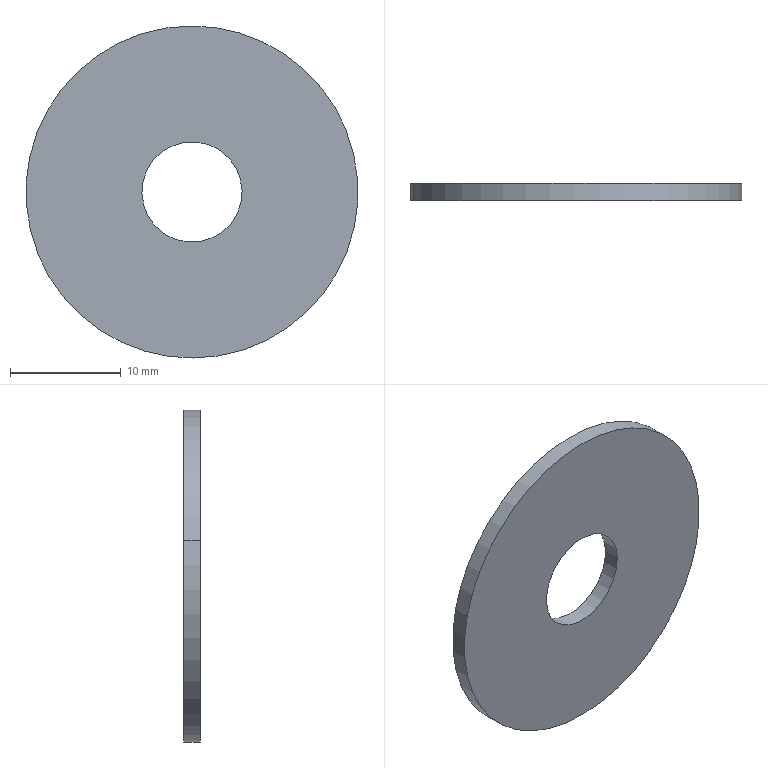Part | STEP file | 2026.6.15-Main Assembly图.sldasm-Part-204 | 1 solid | 6 faces | box 30 x 1.5 x 30 mm | volume 963.585 mm3 | cylinder 4 | plane 2 | commonest cylinder face diameters 9.06 x2 30 x2
STEP:
#1=CARTESIAN_POINT('',(-1645.889,1406.264,3355.366));
#2=VERTEX_POINT('',#1);
#3=CARTESIAN_POINT('',(-1616.588,1406.264,3348.928));
#4=VERTEX_POINT('',#3);
#5=CARTESIAN_POINT('',(-1631.238,1406.264,3352.147));
#6=DIRECTION('',(0.,-1.,0.));
#7=DIRECTION('',(-0.9767,0.,0.2146));
#8=AXIS2_PLACEMENT_3D('',#5,#6,#7);
#9=CIRCLE('',#8,15.);
#10=EDGE_CURVE('',#2,#4,#9,.T.);
#11=ORIENTED_EDGE('',*,*,#10,.F.);
#12=CARTESIAN_POINT('',(-1631.238,1406.264,3352.147));
#13=DIRECTION('',(0.,-1.,0.));
#14=DIRECTION('',(-0.9767,0.,0.2146));
#15=AXIS2_PLACEMENT_3D('',#12,#13,#14);
#16=CIRCLE('',#15,15.);
#17=EDGE_CURVE('',#4,#2,#16,.T.);
#18=ORIENTED_EDGE('',*,*,#17,.F.);
#19=EDGE_LOOP('',(#11,#18));
#20=FACE_OUTER_BOUND('',#19,.T.);
#21=CARTESIAN_POINT('',(-1635.663,1406.264,3353.119));
#22=VERTEX_POINT('',#21);
#23=CARTESIAN_POINT('',(-1626.814,1406.264,3351.175));
#24=VERTEX_POINT('',#23);
#25=CARTESIAN_POINT('',(-1631.238,1406.264,3352.147));
#26=DIRECTION('',(0.,-1.,0.));
#27=DIRECTION('',(-0.9767,0.,0.2146));
#28=AXIS2_PLACEMENT_3D('',#25,#26,#27);
#29=CIRCLE('',#28,4.53);
#30=EDGE_CURVE('',#22,#24,#29,.T.);
#31=ORIENTED_EDGE('',*,*,#30,.T.);
#32=CARTESIAN_POINT('',(-1631.238,1406.264,3352.147));
#33=DIRECTION('',(0.,-1.,0.));
#34=DIRECTION('',(-0.9767,0.,0.2146));
#35=AXIS2_PLACEMENT_3D('',#32,#33,#34);
#36=CIRCLE('',#35,4.53);
#37=EDGE_CURVE('',#24,#22,#36,.T.);
#38=ORIENTED_EDGE('',*,*,#37,.T.);
#39=EDGE_LOOP('',(#31,#38));
#40=FACE_BOUND('',#39,.T.);
#41=CARTESIAN_POINT('',(-1631.238,1406.264,3352.147));
#42=DIRECTION('',(0.,-1.,0.));
#43=DIRECTION('',(0.,0.,-1.));
#44=AXIS2_PLACEMENT_3D('',#41,#42,#43);
#45=PLANE('',#44);
#46=ADVANCED_FACE('',(#20,#40),#45,.F.);
#47=CARTESIAN_POINT('',(-1616.588,1404.764,3348.928));
#48=VERTEX_POINT('',#47);
#49=CARTESIAN_POINT('',(-1616.588,1404.764,3348.928));
#50=DIRECTION('',(0.,-1.,0.));
#51=VECTOR('',#50,1000.);
#52=LINE('',#49,#51);
#53=EDGE_CURVE('',#4,#48,#52,.T.);
#54=ORIENTED_EDGE('',*,*,#53,.T.);
#55=CARTESIAN_POINT('',(-1645.889,1404.764,3355.366));
#56=VERTEX_POINT('',#55);
#57=CARTESIAN_POINT('',(-1631.238,1404.764,3352.147));
#58=DIRECTION('',(0.,-1.,0.));
#59=DIRECTION('',(-0.9767,0.,0.2146));
#60=AXIS2_PLACEMENT_3D('',#57,#58,#59);
#61=CIRCLE('',#60,15.);
#62=EDGE_CURVE('',#56,#48,#61,.T.);
#63=ORIENTED_EDGE('',*,*,#62,.F.);
#64=CARTESIAN_POINT('',(-1645.889,1404.764,3355.366));
#65=DIRECTION('',(0.,-1.,0.));
#66=VECTOR('',#65,1000.);
#67=LINE('',#64,#66);
#68=EDGE_CURVE('',#2,#56,#67,.T.);
#69=ORIENTED_EDGE('',*,*,#68,.F.);
#70=ORIENTED_EDGE('',*,*,#10,.T.);
#71=EDGE_LOOP('',(#54,#63,#69,#70));
#72=FACE_OUTER_BOUND('',#71,.T.);
#73=CARTESIAN_POINT('',(-1631.238,1404.764,3352.147));
#74=DIRECTION('',(0.,1.,0.));
#75=DIRECTION('',(0.9767,0.,-0.2146));
#76=AXIS2_PLACEMENT_3D('',#73,#74,#75);
#77=CYLINDRICAL_SURFACE('',#76,15.);
#78=ADVANCED_FACE('',(#72),#77,.T.);
#79=CARTESIAN_POINT('',(-1626.814,1404.764,3351.175));
#80=VERTEX_POINT('',#79);
#81=CARTESIAN_POINT('',(-1626.814,1404.764,3351.175));
#82=DIRECTION('',(0.,-1.,0.));
#83=VECTOR('',#82,1000.);
#84=LINE('',#81,#83);
#85=EDGE_CURVE('',#24,#80,#84,.T.);
#86=ORIENTED_EDGE('',*,*,#85,.T.);
#87=CARTESIAN_POINT('',(-1635.663,1404.764,3353.119));
#88=VERTEX_POINT('',#87);
#89=CARTESIAN_POINT('',(-1631.238,1404.764,3352.147));
#90=DIRECTION('',(0.,1.,0.));
#91=DIRECTION('',(-0.9767,0.,0.2146));
#92=AXIS2_PLACEMENT_3D('',#89,#90,#91);
#93=CIRCLE('',#92,4.53);
#94=EDGE_CURVE('',#88,#80,#93,.T.);
#95=ORIENTED_EDGE('',*,*,#94,.F.);
#96=CARTESIAN_POINT('',(-1635.663,1404.764,3353.119));
#97=DIRECTION('',(0.,-1.,0.));
#98=VECTOR('',#97,1000.);
#99=LINE('',#96,#98);
#100=EDGE_CURVE('',#22,#88,#99,.T.);
#101=ORIENTED_EDGE('',*,*,#100,.F.);
#102=ORIENTED_EDGE('',*,*,#37,.F.);
#103=EDGE_LOOP('',(#86,#95,#101,#102));
#104=FACE_OUTER_BOUND('',#103,.T.);
#105=CARTESIAN_POINT('',(-1631.238,1404.764,3352.147));
#106=DIRECTION('',(0.,1.,0.));
#107=DIRECTION('',(0.9767,0.,-0.2146));
#108=AXIS2_PLACEMENT_3D('',#105,#106,#107);
#109=CYLINDRICAL_SURFACE('',#108,4.53);
#110=ADVANCED_FACE('',(#104),#109,.F.);
#111=ORIENTED_EDGE('',*,*,#62,.T.);
#112=CARTESIAN_POINT('',(-1631.238,1404.764,3352.147));
#113=DIRECTION('',(0.,-1.,0.));
#114=DIRECTION('',(-0.9767,0.,0.2146));
#115=AXIS2_PLACEMENT_3D('',#112,#113,#114);
#116=CIRCLE('',#115,15.);
#117=EDGE_CURVE('',#48,#56,#116,.T.);
#118=ORIENTED_EDGE('',*,*,#117,.T.);
#119=EDGE_LOOP('',(#111,#118));
#120=FACE_OUTER_BOUND('',#119,.T.);
#121=ORIENTED_EDGE('',*,*,#94,.T.);
#122=CARTESIAN_POINT('',(-1631.238,1404.764,3352.147));
#123=DIRECTION('',(0.,1.,0.));
#124=DIRECTION('',(-0.9767,0.,0.2146));
#125=AXIS2_PLACEMENT_3D('',#122,#123,#124);
#126=CIRCLE('',#125,4.53);
#127=EDGE_CURVE('',#80,#88,#126,.T.);
#128=ORIENTED_EDGE('',*,*,#127,.T.);
#129=EDGE_LOOP('',(#121,#128));
#130=FACE_BOUND('',#129,.T.);
#131=CARTESIAN_POINT('',(-1631.238,1404.764,3352.147));
#132=DIRECTION('',(0.,-1.,0.));
#133=DIRECTION('',(0.,0.,-1.));
#134=AXIS2_PLACEMENT_3D('',#131,#132,#133);
#135=PLANE('',#134);
#136=ADVANCED_FACE('',(#120,#130),#135,.T.);
#137=ORIENTED_EDGE('',*,*,#117,.F.);
#138=ORIENTED_EDGE('',*,*,#53,.F.);
#139=ORIENTED_EDGE('',*,*,#17,.T.);
#140=ORIENTED_EDGE('',*,*,#68,.T.);
#141=EDGE_LOOP('',(#137,#138,#139,#140));
#142=FACE_OUTER_BOUND('',#141,.T.);
#143=CARTESIAN_POINT('',(-1631.238,1404.764,3352.147));
#144=DIRECTION('',(0.,1.,0.));
#145=DIRECTION('',(0.9767,0.,-0.2146));
#146=AXIS2_PLACEMENT_3D('',#143,#144,#145);
#147=CYLINDRICAL_SURFACE('',#146,15.);
#148=ADVANCED_FACE('',(#142),#147,.T.);
#149=ORIENTED_EDGE('',*,*,#127,.F.);
#150=ORIENTED_EDGE('',*,*,#85,.F.);
#151=ORIENTED_EDGE('',*,*,#30,.F.);
#152=ORIENTED_EDGE('',*,*,#100,.T.);
#153=EDGE_LOOP('',(#149,#150,#151,#152));
#154=FACE_OUTER_BOUND('',#153,.T.);
#155=CARTESIAN_POINT('',(-1631.238,1404.764,3352.147));
#156=DIRECTION('',(0.,1.,0.));
#157=DIRECTION('',(0.9767,0.,-0.2146));
#158=AXIS2_PLACEMENT_3D('',#155,#156,#157);
#159=CYLINDRICAL_SURFACE('',#158,4.53);
#160=ADVANCED_FACE('',(#154),#159,.F.);
#161=CLOSED_SHELL('',(#46,#78,#110,#136,#148,#160));
#162=MANIFOLD_SOLID_BREP('',#161);
#163=CARTESIAN_POINT('',(0.,0.,0.));
#164=DIRECTION('',(0.,0.,1.));
#165=DIRECTION('',(1.,0.,0.));
#166=AXIS2_PLACEMENT_3D('',#163,#164,#165);
#167=(LENGTH_UNIT()NAMED_UNIT(*)SI_UNIT(.MILLI.,.METRE.));
#168=UNCERTAINTY_MEASURE_WITH_UNIT(LENGTH_MEASURE(0.00001),#167,'','');
#169=(NAMED_UNIT(*)PLANE_ANGLE_UNIT()SI_UNIT($,.RADIAN.));
#170=(NAMED_UNIT(*)SI_UNIT($,.STERADIAN.)SOLID_ANGLE_UNIT());
#171=(GEOMETRIC_REPRESENTATION_CONTEXT(3)GLOBAL_UNCERTAINTY_ASSIGNED_CONTEXT((#168))GLOBAL_UNIT_ASSIGNED_CONTEXT((#167,#169,#170))REPRESENTATION_CONTEXT('',''));
#172=ADVANCED_BREP_SHAPE_REPRESENTATION('',(#162,#166),#171);